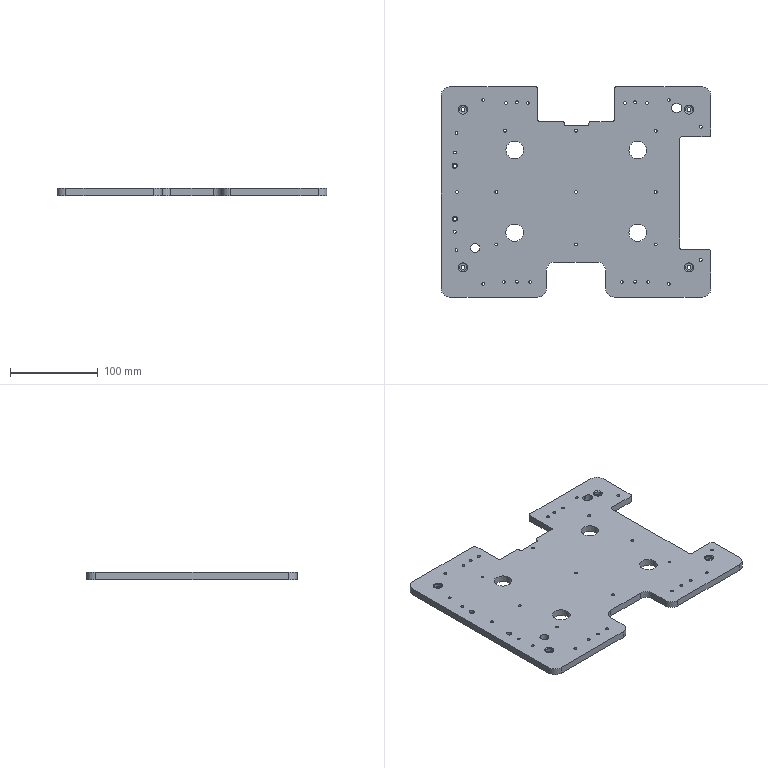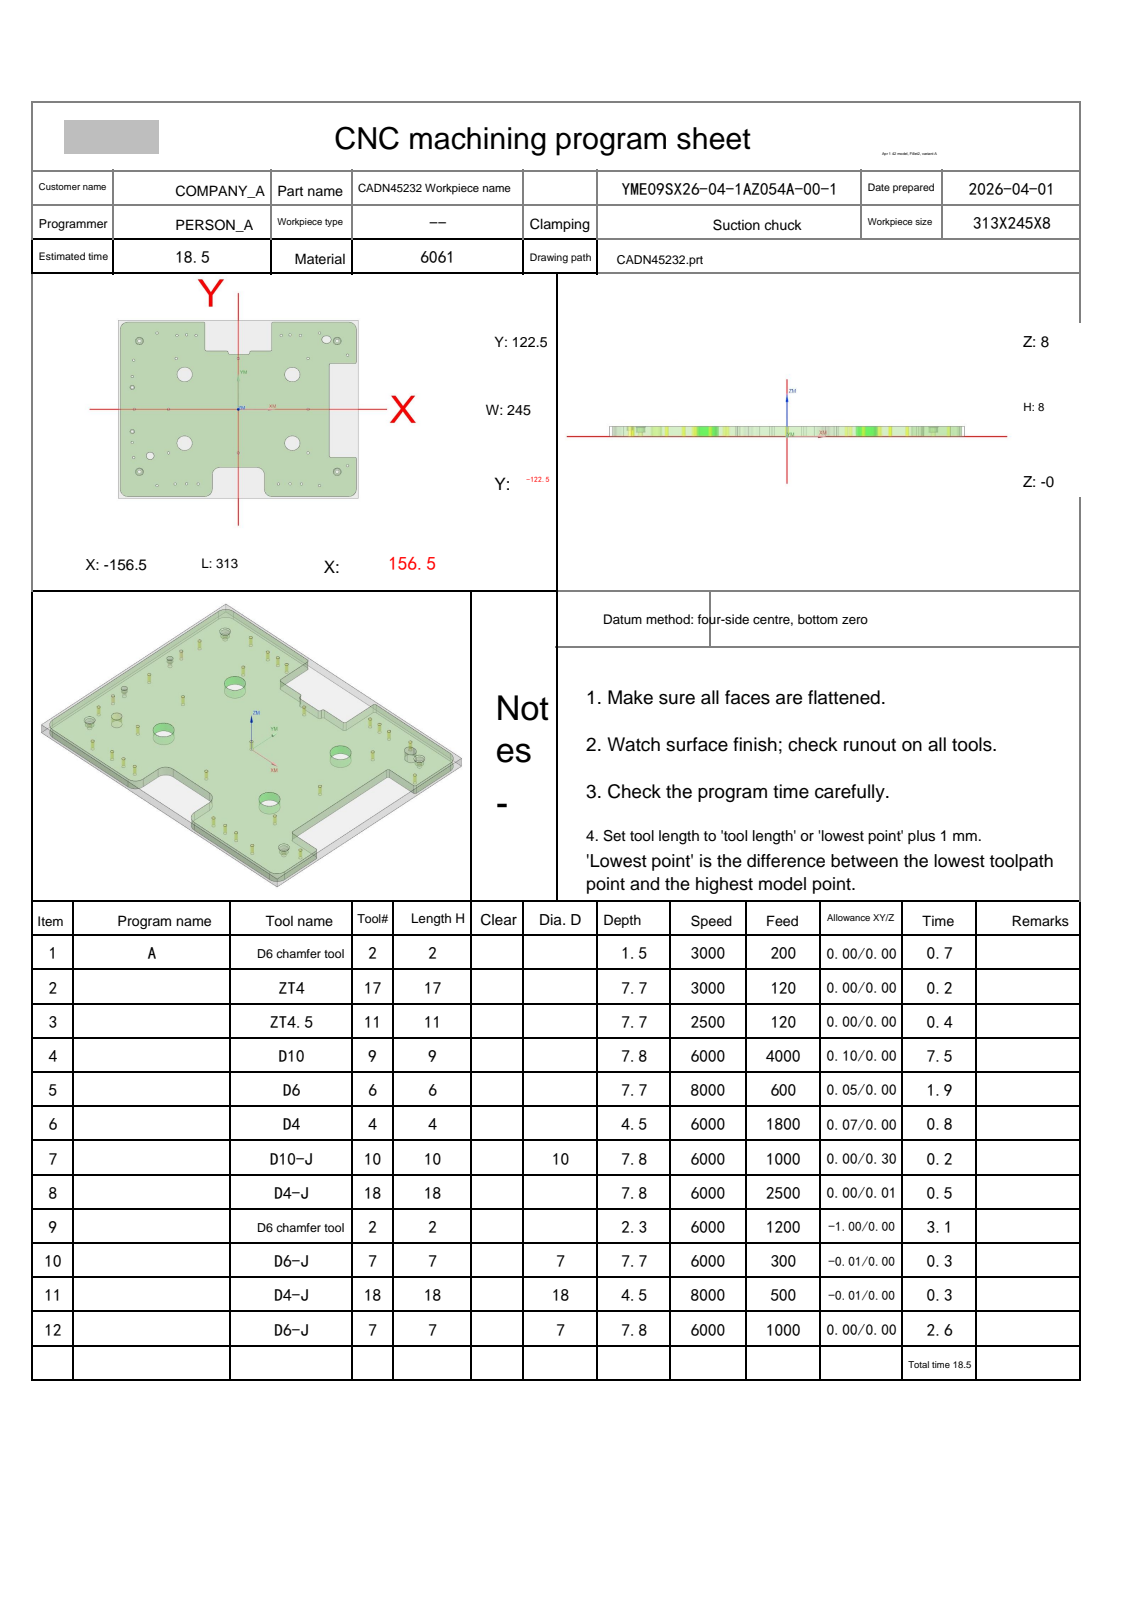NC program | NX | posted by the shop | part box 308 x 240 x 8 mm
Lines 1 to 1898 of 6786, first 1450 of 1896 lines:
%
O0001
(Machine time: 20.76 MIN)
(===Total Tool:9===)
(T2=D6 chamfer tool   D=6.   R=0.   D-  H02 Z=5.7   )
(T17=ZT4    D=4.   DR_a=118 D-  H17 Z=0.3   )
(T11=ZT4.5  D=4.5  DR_a=118 D-  H11 Z=0.3   )
(T9=D10     D=10.  R=0.   D-  H09 Z=0.2   )
(T6=D6      D=6.   R=0.   D-  H06 Z=0.3   )
(T4=D4      D=4.   R=0.   D-  H04 Z=3.5   )
(T10=D10-J  D=10.  R=0.   D10 H10 Z=0.2   )
(T18=D4-J   D=4.   R=0.   D-  H18 Z=0.2   )
(T7=D6-J    D=6.   R=0.   D7  H07 Z=0.2   )
G80 G90 G17 G49 G40
G91 G28 Z0
M01
N1 T02 M06
(D6 chamfer tool  D=6. R=0. H=02 ce=0.00 di=0.00)
G00 G90 G54 X-91. Y0.0 M03 S3000
G43 H02 Z28.
M08
G98 G81 X-91. Y0.0 Z6.5 R9. F200.
X-70.105 Y-46.566
X-91. Y-60.
X-52.35 Y-102.765
X-67.5 Y-102.5
X-82.35 Y-102.765
X-106. Y-105.
X-129. Y-85.991
X-115. Y-63.991
X-136.5 Y-66.5
X-138.327 Y-45.597
Y-30.597
X-135.8 Y0.0
X-138.327 Y30.083
Y45.083
X-136.5 Y67.5
X-129. Y94.009
X-106. Y105.
X-80. Y101.6
X-67.5 Y102.5
X-55. Y101.6
X-81. Y70.
X-70. Y48.
X0.0 Y70.
Y0.0
Y-60.
X52.35 Y-102.765
X67.5 Y-102.5
X82.35 Y-102.765
X106. Y-105.
X129. Y-85.991
X142.5 Y-77.5
X91. Y-60.
X70.458 Y-46.566
X91. Y0.0
X70.458 Y47.847
X91. Y70.
X56. Y101.6
X67.5 Y102.5
X81. Y101.6
X106. Y105.
X129. Y94.009
X142.5 Y74.508
G80
G00 Z28.
G91 G28 Z0.0
M05
M09
G91 G28 Z0.0
M01
N2 T17 M06
(ZT4 D=4. DR_a=118 H=17)
G00 G90 G54 X-138.327 Y30.083 M03 S3000
G43 H17 Z28.
M08
G98 G83 X-138.327 Y30.083 Z.3 R9. F120. Q3.
Y-30.597
G80
G00 Z28.
G91 G28 Z0.0
M05
M09
G91 G28 Z0.0
M01
N3 T11 M06
(ZT4.5 D=4.5 DR_a=118 H=11)
G00 G90 G54 X-129. Y94.009 M03 S2500
G43 H11 Z28.
M08
G98 G83 X-129. Y94.009 Z.3 R9. F120. Q3.
Y-85.991
X129.
Y94.009
G80
G00 Z28.
G91 G28 Z0.0
M05
M09
G91 G28 Z0.0
M01
N4 T09 M06
(D10  D=10. R=0. H=09 ce=0.10 di=0.30)
G00 G90 G54 X70.458 Y-46.566 M03 S6000
G43 H09 Z28.
M08
Z8.5
G03 X72.458 Y-48.566 I2. J0.0 F2700.
X74.458 Y-46.566 I0.0 J2.
X74.458 Y-46.566 Z8.3 I-4. J0.0 F3000.
X74.458 Y-46.566 Z8.1 I-4. J0.0
X74.458 Y-46.566 Z7.9 I-4. J0.0
X74.458 Y-46.566 Z7.7 I-4. J0.0
X74.458 Y-46.566 Z7.5 I-4. J0.0
X74.458 Y-46.566 Z7.3 I-4. J0.0
X74.458 Y-46.566 Z7.1 I-4. J0.0
X74.458 Y-46.566 Z6.9 I-4. J0.0
X74.458 Y-46.566 Z6.7 I-4. J0.0
X74.458 Y-46.566 Z6.5 I-4. J0.0
X74.458 Y-46.566 Z6.3 I-4. J0.0
X74.458 Y-46.566 Z6.1 I-4. J0.0
X74.458 Y-46.566 Z5.9 I-4. J0.0
X74.458 Y-46.566 Z5.7 I-4. J0.0
X74.458 Y-46.566 Z5.5 I-4. J0.0
X74.458 Y-46.566 Z5.3 I-4. J0.0
X74.458 Y-46.566 Z5.1 I-4. J0.0
X74.458 Y-46.566 Z4.9 I-4. J0.0
X74.458 Y-46.566 Z4.7 I-4. J0.0
X74.458 Y-46.566 Z4.5 I-4. J0.0
X74.458 Y-46.566 Z4.3 I-4. J0.0
X74.458 Y-46.566 Z4.1 I-4. J0.0
X74.458 Y-46.566 Z3.9 I-4. J0.0
X74.458 Y-46.566 Z3.7 I-4. J0.0
X74.458 Y-46.566 Z3.5 I-4. J0.0
X74.458 Y-46.566 Z3.3 I-4. J0.0
X74.458 Y-46.566 Z3.1 I-4. J0.0
X74.458 Y-46.566 Z2.9 I-4. J0.0
X74.458 Y-46.566 Z2.7 I-4. J0.0
X74.458 Y-46.566 Z2.5 I-4. J0.0
X74.458 Y-46.566 Z2.3 I-4. J0.0
X74.458 Y-46.566 Z2.1 I-4. J0.0
X74.458 Y-46.566 Z1.9 I-4. J0.0
X74.458 Y-46.566 Z1.7 I-4. J0.0
X74.458 Y-46.566 Z1.5 I-4. J0.0
X74.458 Y-46.566 Z1.3 I-4. J0.0
X74.458 Y-46.566 Z1.1 I-4. J0.0
X74.458 Y-46.566 Z.9 I-4. J0.0
X74.458 Y-46.566 Z.7 I-4. J0.0
X74.458 Y-46.566 Z.5 I-4. J0.0
X74.458 Y-46.566 Z.3 I-4. J0.0
X66.458 Y-46.566 Z.2 I-4. J0.0
X69.894 Y-50.607 I4.094 J0.0
X70.56 Y-50.661 I.666 J4.09
X74.476 Y-47.872 I0.0 J4.144
X74.711 Y-46.478 I-4.03 J1.394
X72.452 Y-42.714 I-4.264 J0.0
X70.378 Y-42.196 I-2.073 J-3.891
X66.858 Y-43.951 I0.0 J-4.409
X65.953 Y-46.654 I3.584 J-2.703
X67.213 Y-49.773 I4.489 J0.0
X70.546 Y-51.188 I3.334 J3.219
X73.206 Y-50.348 I0.0 J4.634
X75.232 Y-46.455 I-2.729 J3.894
X74.722 Y-44.312 I-4.755 J0.0
X70.43 Y-41.671 I-4.292 J-2.167
X68.944 Y-41.906 I0.0 J-4.808
X65.558 Y-46.566 I1.514 J-4.66
X70.458 Y-51.466 I4.9 J0.0
X75.358 Y-46.566 I0.0 J4.9
X70.458 Y-41.666 I-4.9 J0.0
X68.477 Y-42.085 I0.0 J-4.9
X67.018 Y-44.325 I.991 J-2.241
X69.468 Y-46.775 I2.45 J0.0
X70.458 Y-46.566 I0.0 J2.45
G00 Z28.
Y47.847
Z8.5
G03 X72.458 Y45.847 I2. J0.0 F2700.
X74.458 Y47.847 I0.0 J2.
X74.458 Y47.847 Z8.3 I-4. J0.0 F3000.
X74.458 Y47.847 Z8.1 I-4. J0.0
X74.458 Y47.847 Z7.9 I-4. J0.0
X74.458 Y47.847 Z7.7 I-4. J0.0
X74.458 Y47.847 Z7.5 I-4. J0.0
X74.458 Y47.847 Z7.3 I-4. J0.0
X74.458 Y47.847 Z7.1 I-4. J0.0
X74.458 Y47.847 Z6.9 I-4. J0.0
X74.458 Y47.847 Z6.7 I-4. J0.0
X74.458 Y47.847 Z6.5 I-4. J0.0
X74.458 Y47.847 Z6.3 I-4. J0.0
X74.458 Y47.847 Z6.1 I-4. J0.0
X74.458 Y47.847 Z5.9 I-4. J0.0
X74.458 Y47.847 Z5.7 I-4. J0.0
X74.458 Y47.847 Z5.5 I-4. J0.0
X74.458 Y47.847 Z5.3 I-4. J0.0
X74.458 Y47.847 Z5.1 I-4. J0.0
X74.458 Y47.847 Z4.9 I-4. J0.0
X74.458 Y47.847 Z4.7 I-4. J0.0
X74.458 Y47.847 Z4.5 I-4. J0.0
X74.458 Y47.847 Z4.3 I-4. J0.0
X74.458 Y47.847 Z4.1 I-4. J0.0
X74.458 Y47.847 Z3.9 I-4. J0.0
X74.458 Y47.847 Z3.7 I-4. J0.0
X74.458 Y47.847 Z3.5 I-4. J0.0
X74.458 Y47.847 Z3.3 I-4. J0.0
X74.458 Y47.847 Z3.1 I-4. J0.0
X74.458 Y47.847 Z2.9 I-4. J0.0
X74.458 Y47.847 Z2.7 I-4. J0.0
X74.458 Y47.847 Z2.5 I-4. J0.0
X74.458 Y47.847 Z2.3 I-4. J0.0
X74.458 Y47.847 Z2.1 I-4. J0.0
X74.458 Y47.847 Z1.9 I-4. J0.0
X74.458 Y47.847 Z1.7 I-4. J0.0
X74.458 Y47.847 Z1.5 I-4. J0.0
X74.458 Y47.847 Z1.3 I-4. J0.0
X74.458 Y47.847 Z1.1 I-4. J0.0
X74.458 Y47.847 Z.9 I-4. J0.0
X74.458 Y47.847 Z.7 I-4. J0.0
X74.458 Y47.847 Z.5 I-4. J0.0
X74.458 Y47.847 Z.3 I-4. J0.0
X66.458 Y47.847 Z.2 I-4. J0.0
X69.894 Y43.806 I4.094 J0.0
X70.56 Y43.752 I.666 J4.09
X74.476 Y46.541 I0.0 J4.144
X74.711 Y47.935 I-4.03 J1.394
X72.452 Y51.699 I-4.264 J0.0
X70.378 Y52.217 I-2.073 J-3.891
X66.858 Y50.462 I0.0 J-4.409
X65.953 Y47.759 I3.584 J-2.703
X67.213 Y44.64 I4.489 J0.0
X70.546 Y43.225 I3.334 J3.219
X73.206 Y44.065 I0.0 J4.634
X75.232 Y47.958 I-2.729 J3.894
X74.722 Y50.101 I-4.755 J0.0
X70.43 Y52.742 I-4.292 J-2.167
X68.944 Y52.507 I0.0 J-4.808
X65.558 Y47.847 I1.514 J-4.66
X70.458 Y42.947 I4.9 J0.0
X75.358 Y47.847 I0.0 J4.9
X70.458 Y52.747 I-4.9 J0.0
X68.477 Y52.328 I0.0 J-4.9
X67.018 Y50.088 I.991 J-2.241
X69.468 Y47.638 I2.45 J0.0
X70.458 Y47.847 I0.0 J2.45
G00 Z28.
X-70. Y48.
Z8.5
G03 X-68. Y46. I2. J0.0 F2700.
X-66. Y48. I0.0 J2.
X-66. Y48. Z8.3 I-4. J0.0 F3000.
X-66. Y48. Z8.1 I-4. J0.0
X-66. Y48. Z7.9 I-4. J0.0
X-66. Y48. Z7.7 I-4. J0.0
X-66. Y48. Z7.5 I-4. J0.0
X-66. Y48. Z7.3 I-4. J0.0
X-66. Y48. Z7.1 I-4. J0.0
X-66. Y48. Z6.9 I-4. J0.0
X-66. Y48. Z6.7 I-4. J0.0
X-66. Y48. Z6.5 I-4. J0.0
X-66. Y48. Z6.3 I-4. J0.0
X-66. Y48. Z6.1 I-4. J0.0
X-66. Y48. Z5.9 I-4. J0.0
X-66. Y48. Z5.7 I-4. J0.0
X-66. Y48. Z5.5 I-4. J0.0
X-66. Y48. Z5.3 I-4. J0.0
X-66. Y48. Z5.1 I-4. J0.0
X-66. Y48. Z4.9 I-4. J0.0
X-66. Y48. Z4.7 I-4. J0.0
X-66. Y48. Z4.5 I-4. J0.0
X-66. Y48. Z4.3 I-4. J0.0
X-66. Y48. Z4.1 I-4. J0.0
X-66. Y48. Z3.9 I-4. J0.0
X-66. Y48. Z3.7 I-4. J0.0
X-66. Y48. Z3.5 I-4. J0.0
X-66. Y48. Z3.3 I-4. J0.0
X-66. Y48. Z3.1 I-4. J0.0
X-66. Y48. Z2.9 I-4. J0.0
X-66. Y48. Z2.7 I-4. J0.0
X-66. Y48. Z2.5 I-4. J0.0
X-66. Y48. Z2.3 I-4. J0.0
X-66. Y48. Z2.1 I-4. J0.0
X-66. Y48. Z1.9 I-4. J0.0
X-66. Y48. Z1.7 I-4. J0.0
X-66. Y48. Z1.5 I-4. J0.0
X-66. Y48. Z1.3 I-4. J0.0
X-66. Y48. Z1.1 I-4. J0.0
X-66. Y48. Z.9 I-4. J0.0
X-66. Y48. Z.7 I-4. J0.0
X-66. Y48. Z.5 I-4. J0.0
X-66. Y48. Z.3 I-4. J0.0
X-74. Y48. Z.2 I-4. J0.0
X-70.564 Y43.959 I4.094 J0.0
X-69.898 Y43.905 I.666 J4.09
X-65.982 Y46.694 I0.0 J4.144
X-65.748 Y48.088 I-4.03 J1.394
X-68.007 Y51.852 I-4.264 J0.0
X-70.08 Y52.37 I-2.073 J-3.891
X-73.6 Y50.616 I0.0 J-4.409
X-74.505 Y47.912 I3.584 J-2.703
X-73.245 Y44.794 I4.489 J0.0
X-69.912 Y43.379 I3.334 J3.219
X-67.252 Y44.218 I0.0 J4.634
X-65.226 Y48.112 I-2.729 J3.894
X-65.736 Y50.254 I-4.755 J0.0
X-70.028 Y52.896 I-4.292 J-2.167
X-71.514 Y52.66 I0.0 J-4.808
X-74.9 Y48. I1.514 J-4.66
X-70. Y43.1 I4.9 J0.0
X-65.1 Y48. I0.0 J4.9
X-70. Y52.9 I-4.9 J0.0
X-71.981 Y52.482 I0.0 J-4.9
X-73.441 Y50.241 I.991 J-2.241
X-70.991 Y47.791 I2.45 J0.0
X-70. Y48. I0.0 J2.45
G00 Z28.
X-70.105 Y-46.566
Z8.5
G03 X-68.105 Y-48.566 I2. J0.0 F2700.
X-66.105 Y-46.566 I0.0 J2.
X-66.105 Y-46.566 Z8.3 I-4. J0.0 F3000.
X-66.105 Y-46.566 Z8.1 I-4. J0.0
X-66.105 Y-46.566 Z7.9 I-4. J0.0
X-66.105 Y-46.566 Z7.7 I-4. J0.0
X-66.105 Y-46.566 Z7.5 I-4. J0.0
X-66.105 Y-46.566 Z7.3 I-4. J0.0
X-66.105 Y-46.566 Z7.1 I-4. J0.0
X-66.105 Y-46.566 Z6.9 I-4. J0.0
X-66.105 Y-46.566 Z6.7 I-4. J0.0
X-66.105 Y-46.566 Z6.5 I-4. J0.0
X-66.105 Y-46.566 Z6.3 I-4. J0.0
X-66.105 Y-46.566 Z6.1 I-4. J0.0
X-66.105 Y-46.566 Z5.9 I-4. J0.0
X-66.105 Y-46.566 Z5.7 I-4. J0.0
X-66.105 Y-46.566 Z5.5 I-4. J0.0
X-66.105 Y-46.566 Z5.3 I-4. J0.0
X-66.105 Y-46.566 Z5.1 I-4. J0.0
X-66.105 Y-46.566 Z4.9 I-4. J0.0
X-66.105 Y-46.566 Z4.7 I-4. J0.0
X-66.105 Y-46.566 Z4.5 I-4. J0.0
X-66.105 Y-46.566 Z4.3 I-4. J0.0
X-66.105 Y-46.566 Z4.1 I-4. J0.0
X-66.105 Y-46.566 Z3.9 I-4. J0.0
X-66.105 Y-46.566 Z3.7 I-4. J0.0
X-66.105 Y-46.566 Z3.5 I-4. J0.0
X-66.105 Y-46.566 Z3.3 I-4. J0.0
X-66.105 Y-46.566 Z3.1 I-4. J0.0
X-66.105 Y-46.566 Z2.9 I-4. J0.0
X-66.105 Y-46.566 Z2.7 I-4. J0.0
X-66.105 Y-46.566 Z2.5 I-4. J0.0
X-66.105 Y-46.566 Z2.3 I-4. J0.0
X-66.105 Y-46.566 Z2.1 I-4. J0.0
X-66.105 Y-46.566 Z1.9 I-4. J0.0
X-66.105 Y-46.566 Z1.7 I-4. J0.0
X-66.105 Y-46.566 Z1.5 I-4. J0.0
X-66.105 Y-46.566 Z1.3 I-4. J0.0
X-66.105 Y-46.566 Z1.1 I-4. J0.0
X-66.105 Y-46.566 Z.9 I-4. J0.0
X-66.105 Y-46.566 Z.7 I-4. J0.0
X-66.105 Y-46.566 Z.5 I-4. J0.0
X-66.105 Y-46.566 Z.3 I-4. J0.0
X-74.105 Y-46.566 Z.2 I-4. J0.0
X-70.669 Y-50.607 I4.094 J0.0
X-70.003 Y-50.661 I.666 J4.09
X-66.087 Y-47.872 I0.0 J4.144
X-65.852 Y-46.478 I-4.03 J1.394
X-68.111 Y-42.714 I-4.264 J0.0
X-70.185 Y-42.196 I-2.073 J-3.891
X-73.705 Y-43.951 I0.0 J-4.409
X-74.61 Y-46.654 I3.584 J-2.703
X-73.35 Y-49.773 I4.489 J0.0
X-70.017 Y-51.188 I3.334 J3.219
X-67.357 Y-50.348 I0.0 J4.634
X-65.331 Y-46.455 I-2.729 J3.894
X-65.841 Y-44.312 I-4.755 J0.0
X-70.133 Y-41.671 I-4.292 J-2.167
X-71.619 Y-41.906 I0.0 J-4.808
X-75.005 Y-46.566 I1.514 J-4.66
X-70.105 Y-51.466 I4.9 J0.0
X-65.205 Y-46.566 I0.0 J4.9
X-70.105 Y-41.666 I-4.9 J0.0
X-72.086 Y-42.085 I0.0 J-4.9
X-73.545 Y-44.325 I.991 J-2.241
X-71.095 Y-46.775 I2.45 J0.0
X-70.105 Y-46.566 I0.0 J2.45
G00 Z28.
G00 G90 X-159.1 Y0.0 M03 S6000
Z28.
Z8.5
G01 Y110. Z8.461 F4000.
G02 X-144. Y125.1 Z8.452 I15.1 J0.0
G01 X-45.5 Z8.417
G02 X-38.4 Y118. Z8.413 I0.0 J-7.1
G01 Y85.389 Z8.401
X-14.961 Z8.393
X-13.8 Y85.272 Z8.392
X-12.44 Y84.851
X-11.191 Y84.169 Z8.391
X-10.103 Y83.251
X-9.219 Y82.136 Z8.39
X-8.574 Y80.868
X-8.557 Y80.806
X10.141 Z8.383
X10.221 Y81.063
X10.903 Y82.312
X11.82 Y83.401 Z8.382
X12.935 Y84.285
X14.203 Y84.931 Z8.381
X15.538 Y85.301
X16.566 Y85.389 Z8.38
X38.4 Z8.372
Y118. Z8.361
G02 X45.5 Y125.1 Z8.357 I7.1 J0.0
G01 X144. Z8.322
G02 X159.1 Y110. Z8.313 I0.0 J-15.1
G01 Y65.004 Z8.297
G02 X152. Y57.904 Z8.293 I-7.1 J0.0
G01 X123.763 Z8.283
Y-60.896 Z8.24
X152. Z8.23
G02 X159.1 Y-67.996 Z8.226 I0.0 J-7.1
G01 Y-110. Z8.211
G02 X144. Y-125.1 Z8.203 I-15.1 J0.0
G01 X44. Z8.167
G02 X28.9 Y-110. Z8.158 I0.0 J15.1
G01 Y-90. Z8.151
G03 X24. Y-85.1 Z8.149 I-4.9 J0.0
G01 X-24. Z8.131
G03 X-28.9 Y-90. Z8.129 I0.0 J-4.9
G01 Y-110. Z8.122
G02 X-44. Y-125.1 Z8.113 I-15.1 J0.0
G01 X-144. Z8.077
G02 X-159.1 Y-110. Z8.069 I0.0 J15.1
G01 Y110. Z7.99
G02 X-144. Y125.1 Z7.982 I15.1 J0.0
G01 X-45.5 Z7.946
G02 X-38.4 Y118. Z7.942 I0.0 J-7.1
G01 Y85.389 Z7.931
X-14.961 Z7.922
X-13.8 Y85.272
X-12.44 Y84.851 Z7.921
X-11.191 Y84.169
X-10.103 Y83.251 Z7.92
X-9.219 Y82.136
X-8.574 Y80.868 Z7.919
X-8.557 Y80.806
X10.141 Z7.913
X10.221 Y81.063
X10.903 Y82.312 Z7.912
X11.82 Y83.401
X12.935 Y84.285 Z7.911
X14.203 Y84.931 Z7.91
X15.538 Y85.301
X16.566 Y85.389
X38.4 Z7.902
Y118. Z7.89
G02 X45.5 Y125.1 Z7.886 I7.1 J0.0
G01 X144. Z7.851
G02 X159.1 Y110. Z7.842 I0.0 J-15.1
G01 Y65.004 Z7.826
G02 X152. Y57.904 Z7.822 I-7.1 J0.0
G01 X123.763 Z7.812
Y-60.896 Z7.77
X152. Z7.76
G02 X159.1 Y-67.996 Z7.756 I0.0 J-7.1
G01 Y-110. Z7.741
G02 X144. Y-125.1 Z7.732 I-15.1 J0.0
G01 X44. Z7.696
G02 X28.9 Y-110. Z7.688 I0.0 J15.1
G01 Y-90. Z7.681
G03 X24. Y-85.1 Z7.678 I-4.9 J0.0
G01 X-24. Z7.661
G03 X-28.9 Y-90. Z7.658 I0.0 J-4.9
G01 Y-110. Z7.651
G02 X-44. Y-125.1 Z7.642 I-15.1 J0.0
G01 X-144. Z7.607
G02 X-159.1 Y-110. Z7.598 I0.0 J15.1
G01 Y110. Z7.519
G02 X-144. Y125.1 Z7.511 I15.1 J0.0
G01 X-45.5 Z7.476
G02 X-38.4 Y118. Z7.472 I0.0 J-7.1
G01 Y85.389 Z7.46
X-14.961 Z7.452
X-13.8 Y85.272 Z7.451
X-12.44 Y84.851
X-11.191 Y84.169 Z7.45
X-10.103 Y83.251
X-9.219 Y82.136 Z7.449
X-8.574 Y80.868
X-8.557 Y80.806
X10.141 Z7.442
X10.221 Y81.063
X10.903 Y82.312 Z7.441
X11.82 Y83.401
X12.935 Y84.285 Z7.44
X14.203 Y84.931
X15.538 Y85.301 Z7.439
X16.566 Y85.389
X38.4 Z7.431
Y118. Z7.42
G02 X45.5 Y125.1 Z7.416 I7.1 J0.0
G01 X144. Z7.38
G02 X159.1 Y110. Z7.372 I0.0 J-15.1
G01 Y65.004 Z7.356
G02 X152. Y57.904 Z7.352 I-7.1 J0.0
G01 X123.763 Z7.342
Y-60.896 Z7.299
X152. Z7.289
G02 X159.1 Y-67.996 Z7.285 I0.0 J-7.1
G01 Y-110. Z7.27
G02 X144. Y-125.1 Z7.262 I-15.1 J0.0
G01 X44. Z7.226
G02 X28.9 Y-110. Z7.217 I0.0 J15.1
G01 Y-90. Z7.21
G03 X24. Y-85.1 Z7.207 I-4.9 J0.0
G01 X-24. Z7.19
G03 X-28.9 Y-90. Z7.187 I0.0 J-4.9
G01 Y-110. Z7.18
G02 X-44. Y-125.1 Z7.172 I-15.1 J0.0
G01 X-144. Z7.136
G02 X-159.1 Y-110. Z7.128 I0.0 J15.1
G01 Y110. Z7.049
G02 X-144. Y125.1 Z7.04 I15.1 J0.0
G01 X-45.5 Z7.005
G02 X-38.4 Y118. Z7.001 I0.0 J-7.1
G01 Y85.389 Z6.99
X-14.961 Z6.981
X-13.8 Y85.272
X-12.44 Y84.851 Z6.98
X-11.191 Y84.169
X-10.103 Y83.251 Z6.979
X-9.219 Y82.136
X-8.574 Y80.868 Z6.978
X-8.557 Y80.806
X10.141 Z6.971
X10.221 Y81.063
X10.903 Y82.312
X11.82 Y83.401 Z6.97
X12.935 Y84.285
X14.203 Y84.931 Z6.969
X15.538 Y85.301
X16.566 Y85.389 Z6.968
X38.4 Z6.961
Y118. Z6.949
G02 X45.5 Y125.1 Z6.945 I7.1 J0.0
G01 X144. Z6.91
G02 X159.1 Y110. Z6.901 I0.0 J-15.1
G01 Y65.004 Z6.885
G02 X152. Y57.904 Z6.881 I-7.1 J0.0
G01 X123.763 Z6.871
Y-60.896 Z6.829
X152. Z6.818
G02 X159.1 Y-67.996 Z6.814 I0.0 J-7.1
G01 Y-110. Z6.799
G02 X144. Y-125.1 Z6.791 I-15.1 J0.0
G01 X44. Z6.755
G02 X28.9 Y-110. Z6.747 I0.0 J15.1
G01 Y-90. Z6.74
G03 X24. Y-85.1 Z6.737 I-4.9 J0.0
G01 X-24. Z6.72
G03 X-28.9 Y-90. Z6.717 I0.0 J-4.9
G01 Y-110. Z6.71
G02 X-44. Y-125.1 Z6.701 I-15.1 J0.0
G01 X-144. Z6.665
G02 X-159.1 Y-110. Z6.657 I0.0 J15.1
G01 Y110. Z6.578
G02 X-144. Y125.1 Z6.57 I15.1 J0.0
G01 X-45.5 Z6.535
G02 X-38.4 Y118. Z6.531 I0.0 J-7.1
G01 Y85.389 Z6.519
X-14.961 Z6.511
X-13.8 Y85.272 Z6.51
X-12.44 Y84.851
X-11.191 Y84.169 Z6.509
X-10.103 Y83.251
X-9.219 Y82.136 Z6.508
X-8.574 Y80.868
X-8.557 Y80.806
X10.141 Z6.501
X10.221 Y81.063
X10.903 Y82.312 Z6.5
X11.82 Y83.401
X12.935 Y84.285 Z6.499
X14.203 Y84.931
X15.538 Y85.301 Z6.498
X16.566 Y85.389
X38.4 Z6.49
Y118. Z6.478
G02 X45.5 Y125.1 Z6.474 I7.1 J0.0
G01 X144. Z6.439
G02 X159.1 Y110. Z6.431 I0.0 J-15.1
G01 Y65.004 Z6.415
G02 X152. Y57.904 Z6.411 I-7.1 J0.0
G01 X123.763 Z6.4
Y-60.896 Z6.358
X152. Z6.348
G02 X159.1 Y-67.996 Z6.344 I0.0 J-7.1
G01 Y-110. Z6.329
G02 X144. Y-125.1 Z6.32 I-15.1 J0.0
G01 X44. Z6.285
G02 X28.9 Y-110. Z6.276 I0.0 J15.1
G01 Y-90. Z6.269
G03 X24. Y-85.1 Z6.266 I-4.9 J0.0
G01 X-24. Z6.249
G03 X-28.9 Y-90. Z6.246 I0.0 J-4.9
G01 Y-110. Z6.239
G02 X-44. Y-125.1 Z6.231 I-15.1 J0.0
G01 X-144. Z6.195
G02 X-159.1 Y-110. Z6.186 I0.0 J15.1
G01 Y110. Z6.108
G02 X-144. Y125.1 Z6.099 I15.1 J0.0
G01 X-45.5 Z6.064
G02 X-38.4 Y118. Z6.06 I0.0 J-7.1
G01 Y85.389 Z6.048
X-14.961 Z6.04
X-13.8 Y85.272
X-12.44 Y84.851 Z6.039
X-11.191 Y84.169
X-10.103 Y83.251 Z6.038
X-9.219 Y82.136 Z6.037
X-8.574 Y80.868
X-8.557 Y80.806
X10.141 Z6.03
X10.221 Y81.063
X10.903 Y82.312
X11.82 Y83.401 Z6.029
X12.935 Y84.285
X14.203 Y84.931 Z6.028
X15.538 Y85.301
X16.566 Y85.389 Z6.027
X38.4 Z6.019
Y118. Z6.008
G02 X45.5 Y125.1 Z6.004 I7.1 J0.0
G01 X144. Z5.969
G02 X159.1 Y110. Z5.96 I0.0 J-15.1
G01 Y65.004 Z5.944
G02 X152. Y57.904 Z5.94 I-7.1 J0.0
G01 X123.763 Z5.93
Y-60.896 Z5.887
X152. Z5.877
G02 X159.1 Y-67.996 Z5.873 I0.0 J-7.1
G01 Y-110. Z5.858
G02 X144. Y-125.1 Z5.85 I-15.1 J0.0
G01 X44. Z5.814
G02 X28.9 Y-110. Z5.806 I0.0 J15.1
G01 Y-90. Z5.798
G03 X24. Y-85.1 Z5.796 I-4.9 J0.0
G01 X-24. Z5.778
G03 X-28.9 Y-90. Z5.776 I0.0 J-4.9
G01 Y-110. Z5.769
G02 X-44. Y-125.1 Z5.76 I-15.1 J0.0
G01 X-144. Z5.724
G02 X-159.1 Y-110. Z5.716 I0.0 J15.1
G01 Y110. Z5.637
G02 X-144. Y125.1 Z5.629 I15.1 J0.0
G01 X-45.5 Z5.593
G02 X-38.4 Y118. Z5.589 I0.0 J-7.1
G01 Y85.389 Z5.578
X-14.961 Z5.569
X-13.8 Y85.272
X-12.44 Y84.851 Z5.568
X-11.191 Y84.169
X-10.103 Y83.251 Z5.567
X-9.219 Y82.136
X-8.574 Y80.868 Z5.566
X-8.557 Y80.806
X10.141 Z5.56
X10.221 Y81.063
X10.903 Y82.312 Z5.559
X11.82 Y83.401
X12.935 Y84.285 Z5.558
X14.203 Y84.931
X15.538 Y85.301 Z5.557
X16.566 Y85.389
X38.4 Z5.549
Y118. Z5.537
G02 X45.5 Y125.1 Z5.533 I7.1 J0.0
G01 X144. Z5.498
G02 X159.1 Y110. Z5.49 I0.0 J-15.1
G01 Y65.004 Z5.473
G02 X152. Y57.904 Z5.469 I-7.1 J0.0
G01 X123.763 Z5.459
Y-60.896 Z5.417
X152. Z5.407
G02 X159.1 Y-67.996 Z5.403 I0.0 J-7.1
G01 Y-110. Z5.388
G02 X144. Y-125.1 Z5.379 I-15.1 J0.0
G01 X44. Z5.343
G02 X28.9 Y-110. Z5.335 I0.0 J15.1
G01 Y-90. Z5.328
G03 X24. Y-85.1 Z5.325 I-4.9 J0.0
G01 X-24. Z5.308
G03 X-28.9 Y-90. Z5.305 I0.0 J-4.9
G01 Y-110. Z5.298
G02 X-44. Y-125.1 Z5.289 I-15.1 J0.0
G01 X-144. Z5.254
G02 X-159.1 Y-110. Z5.245 I0.0 J15.1
G01 Y110. Z5.167
G02 X-144. Y125.1 Z5.158 I15.1 J0.0
G01 X-45.5 Z5.123
G02 X-38.4 Y118. Z5.119 I0.0 J-7.1
G01 Y85.389 Z5.107
X-14.961 Z5.099
X-13.8 Y85.272 Z5.098
X-12.44 Y84.851
X-11.191 Y84.169 Z5.097
X-10.103 Y83.251
X-9.219 Y82.136 Z5.096
X-8.574 Y80.868
X-8.557 Y80.806
X10.141 Z5.089
X10.221 Y81.063
X10.903 Y82.312 Z5.088
X11.82 Y83.401
X12.935 Y84.285 Z5.087
X14.203 Y84.931
X15.538 Y85.301 Z5.086
X16.566 Y85.389
X38.4 Z5.078
Y118. Z5.067
G02 X45.5 Y125.1 Z5.063 I7.1 J0.0
G01 X144. Z5.027
G02 X159.1 Y110. Z5.019 I0.0 J-15.1
G01 Y65.004 Z5.003
G02 X152. Y57.904 Z4.999 I-7.1 J0.0
G01 X123.763 Z4.989
Y-60.896 Z4.946
X152. Z4.936
G02 X159.1 Y-67.996 Z4.932 I0.0 J-7.1
G01 Y-110. Z4.917
G02 X144. Y-125.1 Z4.909 I-15.1 J0.0
G01 X44. Z4.873
G02 X28.9 Y-110. Z4.864 I0.0 J15.1
G01 Y-90. Z4.857
G03 X24. Y-85.1 Z4.854 I-4.9 J0.0
G01 X-24. Z4.837
G03 X-28.9 Y-90. Z4.835 I0.0 J-4.9
G01 Y-110. Z4.827
G02 X-44. Y-125.1 Z4.819 I-15.1 J0.0
G01 X-144. Z4.783
G02 X-159.1 Y-110. Z4.775 I0.0 J15.1
G01 Y110. Z4.696
G02 X-144. Y125.1 Z4.687 I15.1 J0.0
G01 X-45.5 Z4.652
G02 X-38.4 Y118. Z4.648 I0.0 J-7.1
G01 Y85.389 Z4.637
X-14.961 Z4.628
X-13.8 Y85.272
X-12.44 Y84.851 Z4.627
X-11.191 Y84.169
X-10.103 Y83.251 Z4.626
X-9.219 Y82.136
X-8.574 Y80.868 Z4.625
X-8.557 Y80.806
X10.141 Z4.619
X10.221 Y81.063 Z4.618
X10.903 Y82.312
X11.82 Y83.401 Z4.617
X12.935 Y84.285
X14.203 Y84.931 Z4.616
X15.538 Y85.301
X16.566 Y85.389
X38.4 Z4.608
Y118. Z4.596
G02 X45.5 Y125.1 Z4.592 I7.1 J0.0
G01 X144. Z4.557
G02 X159.1 Y110. Z4.548 I0.0 J-15.1
G01 Y65.004 Z4.532
G02 X152. Y57.904 Z4.528 I-7.1 J0.0
G01 X123.763 Z4.518
Y-60.896 Z4.476
X152. Z4.466
G02 X159.1 Y-67.996 Z4.462 I0.0 J-7.1
G01 Y-110. Z4.447
G02 X144. Y-125.1 Z4.438 I-15.1 J0.0
G01 X44. Z4.402
G02 X28.9 Y-110. Z4.394 I0.0 J15.1
G01 Y-90. Z4.387
G03 X24. Y-85.1 Z4.384 I-4.9 J0.0
G01 X-24. Z4.367
G03 X-28.9 Y-90. Z4.364 I0.0 J-4.9
G01 Y-110. Z4.357
G02 X-44. Y-125.1 Z4.348 I-15.1 J0.0
G01 X-144. Z4.313
G02 X-159.1 Y-110. Z4.304 I0.0 J15.1
G01 Y110. Z4.225
G02 X-144. Y125.1 Z4.217 I15.1 J0.0
G01 X-45.5 Z4.182
G02 X-38.4 Y118. Z4.178 I0.0 J-7.1
G01 Y85.389 Z4.166
X-14.961 Z4.158
X-13.8 Y85.272 Z4.157
X-12.44 Y84.851
X-11.191 Y84.169 Z4.156
X-10.103 Y83.251
X-9.219 Y82.136 Z4.155
X-8.574 Y80.868
X-8.557 Y80.806
X10.141 Z4.148
X10.221 Y81.063
X10.903 Y82.312 Z4.147
X11.82 Y83.401
X12.935 Y84.285 Z4.146
X14.203 Y84.931
X15.538 Y85.301 Z4.145
X16.566 Y85.389
X38.4 Z4.137
Y118. Z4.125
G02 X45.5 Y125.1 Z4.121 I7.1 J0.0
G01 X144. Z4.086
G02 X159.1 Y110. Z4.078 I0.0 J-15.1
G01 Y65.004 Z4.062
G02 X152. Y57.904 Z4.058 I-7.1 J0.0
G01 X123.763 Z4.048
Y-60.896 Z4.005
X152. Z3.995
G02 X159.1 Y-67.996 Z3.991 I0.0 J-7.1
G01 Y-110. Z3.976
G02 X144. Y-125.1 Z3.967 I-15.1 J0.0
G01 X44. Z3.932
G02 X28.9 Y-110. Z3.923 I0.0 J15.1
G01 Y-90. Z3.916
G03 X24. Y-85.1 Z3.913 I-4.9 J0.0
G01 X-24. Z3.896
G03 X-28.9 Y-90. Z3.893 I0.0 J-4.9
G01 Y-110. Z3.886
G02 X-44. Y-125.1 Z3.878 I-15.1 J0.0
G01 X-144. Z3.842
G02 X-159.1 Y-110. Z3.833 I0.0 J15.1
G01 Y110. Z3.755
G02 X-144. Y125.1 Z3.746 I15.1 J0.0
G01 X-45.5 Z3.711
G02 X-38.4 Y118. Z3.707 I0.0 J-7.1
G01 Y85.389 Z3.695
X-14.961 Z3.687
X-13.8 Y85.272
X-12.44 Y84.851 Z3.686
X-11.191 Y84.169
X-10.103 Y83.251 Z3.685
X-9.219 Y82.136
X-8.574 Y80.868 Z3.684
X-8.557 Y80.806
X10.141 Z3.677
X10.221 Y81.063
X10.903 Y82.312
X11.82 Y83.401 Z3.676
X12.935 Y84.285
X14.203 Y84.931 Z3.675
X15.538 Y85.301
X16.566 Y85.389 Z3.674
X38.4 Z3.667
Y118. Z3.655
G02 X45.5 Y125.1 Z3.651 I7.1 J0.0
G01 X144. Z3.616
G02 X159.1 Y110. Z3.607 I0.0 J-15.1
G01 Y65.004 Z3.591
G02 X152. Y57.904 Z3.587 I-7.1 J0.0
G01 X123.763 Z3.577
Y-60.896 Z3.534
X152. Z3.524
G02 X159.1 Y-67.996 Z3.52 I0.0 J-7.1
G01 Y-110. Z3.505
G02 X144. Y-125.1 Z3.497 I-15.1 J0.0
G01 X44. Z3.461
G02 X28.9 Y-110. Z3.453 I0.0 J15.1
G01 Y-90. Z3.445
G03 X24. Y-85.1 Z3.443 I-4.9 J0.0
G01 X-24. Z3.426
G03 X-28.9 Y-90. Z3.423 I0.0 J-4.9
G01 Y-110. Z3.416
G02 X-44. Y-125.1 Z3.407 I-15.1 J0.0
G01 X-144. Z3.371
G02 X-159.1 Y-110. Z3.363 I0.0 J15.1
G01 Y110. Z3.284
G02 X-144. Y125.1 Z3.276 I15.1 J0.0
G01 X-45.5 Z3.24
G02 X-38.4 Y118. Z3.236 I0.0 J-7.1
G01 Y85.389 Z3.225
X-14.961 Z3.216
X-13.8 Y85.272
X-12.44 Y84.851 Z3.215
X-11.191 Y84.169
X-10.103 Y83.251 Z3.214
X-9.219 Y82.136
X-8.574 Y80.868 Z3.213
X-8.557 Y80.806
X10.141 Z3.207
X10.221 Y81.063
X10.903 Y82.312 Z3.206
X11.82 Y83.401
X12.935 Y84.285 Z3.205
X14.203 Y84.931
X15.538 Y85.301 Z3.204
X16.566 Y85.389
X38.4 Z3.196
Y118. Z3.184
G02 X45.5 Y125.1 Z3.18 I7.1 J0.0
G01 X144. Z3.145
G02 X159.1 Y110. Z3.137 I0.0 J-15.1
G01 Y65.004 Z3.12
G02 X152. Y57.904 Z3.116 I-7.1 J0.0
G01 X123.763 Z3.106
Y-60.896 Z3.064
X152. Z3.054
G02 X159.1 Y-67.996 Z3.05 I0.0 J-7.1
G01 Y-110. Z3.035
G02 X144. Y-125.1 Z3.026 I-15.1 J0.0
G01 X44. Z2.991
G02 X28.9 Y-110. Z2.982 I0.0 J15.1
G01 Y-90. Z2.975
G03 X24. Y-85.1 Z2.972 I-4.9 J0.0
G01 X-24. Z2.955
G03 X-28.9 Y-90. Z2.952 I0.0 J-4.9
G01 Y-110. Z2.945
G02 X-44. Y-125.1 Z2.937 I-15.1 J0.0
G01 X-144. Z2.901
G02 X-159.1 Y-110. Z2.892 I0.0 J15.1
G01 Y110. Z2.814
G02 X-144. Y125.1 Z2.805 I15.1 J0.0
G01 X-45.5 Z2.77
G02 X-38.4 Y118. Z2.766 I0.0 J-7.1
G01 Y85.389 Z2.754
X-14.961 Z2.746
X-13.8 Y85.272 Z2.745
X-12.44 Y84.851
X-11.191 Y84.169 Z2.744
X-10.103 Y83.251
X-9.219 Y82.136 Z2.743
X-8.574 Y80.868
X-8.557 Y80.806
X10.141 Z2.736
X10.221 Y81.063
X10.903 Y82.312
X11.82 Y83.401 Z2.735
X12.935 Y84.285
X14.203 Y84.931 Z2.734
X15.538 Y85.301
X16.566 Y85.389 Z2.733
X38.4 Z2.725
Y118. Z2.714
G02 X45.5 Y125.1 Z2.71 I7.1 J0.0
G01 X144. Z2.674
G02 X159.1 Y110. Z2.666 I0.0 J-15.1
G01 Y65.004 Z2.65
G02 X152. Y57.904 Z2.646 I-7.1 J0.0
G01 X123.763 Z2.636
Y-60.896 Z2.593
X152. Z2.583
G02 X159.1 Y-67.996 Z2.579 I0.0 J-7.1
G01 Y-110. Z2.564
G02 X144. Y-125.1 Z2.556 I-15.1 J0.0
G01 X44. Z2.52
G02 X28.9 Y-110. Z2.511 I0.0 J15.1
G01 Y-90. Z2.504
G03 X24. Y-85.1 Z2.502 I-4.9 J0.0
G01 X-24. Z2.484
G03 X-28.9 Y-90. Z2.482 I0.0 J-4.9
G01 Y-110. Z2.474
G02 X-44. Y-125.1 Z2.466 I-15.1 J0.0
G01 X-144. Z2.43
G02 X-159.1 Y-110. Z2.422 I0.0 J15.1
G01 Y110. Z2.343
G02 X-144. Y125.1 Z2.335 I15.1 J0.0
G01 X-45.5 Z2.299
G02 X-38.4 Y118. Z2.295 I0.0 J-7.1
G01 Y85.389 Z2.284
X-14.961 Z2.275
X-13.8 Y85.272
X-12.44 Y84.851 Z2.274
X-11.191 Y84.169
X-10.103 Y83.251 Z2.273
X-9.219 Y82.136
X-8.574 Y80.868 Z2.272
X-8.557 Y80.806
X10.141 Z2.266
X10.221 Y81.063 Z2.265
X10.903 Y82.312
X11.82 Y83.401 Z2.264
X12.935 Y84.285
X14.203 Y84.931 Z2.263
X15.538 Y85.301
X16.566 Y85.389
X38.4 Z2.255
Y118. Z2.243
G02 X45.5 Y125.1 Z2.239 I7.1 J0.0
G01 X144. Z2.204
G02 X159.1 Y110. Z2.195 I0.0 J-15.1
G01 Y65.004 Z2.179
G02 X152. Y57.904 Z2.175 I-7.1 J0.0
G01 X123.763 Z2.165
Y-60.896 Z2.123
X152. Z2.113
G02 X159.1 Y-67.996 Z2.109 I0.0 J-7.1
G01 Y-110. Z2.094
G02 X144. Y-125.1 Z2.085 I-15.1 J0.0
G01 X44. Z2.049
G02 X28.9 Y-110. Z2.041 I0.0 J15.1
G01 Y-90. Z2.034
G03 X24. Y-85.1 Z2.031 I-4.9 J0.0
G01 X-24. Z2.014
G03 X-28.9 Y-90. Z2.011 I0.0 J-4.9
G01 Y-110. Z2.004
G02 X-44. Y-125.1 Z1.995 I-15.1 J0.0
G01 X-144. Z1.96
G02 X-159.1 Y-110. Z1.951 I0.0 J15.1
G01 Y110. Z1.872
G02 X-144. Y125.1 Z1.864 I15.1 J0.0
G01 X-45.5 Z1.829
G02 X-38.4 Y118. Z1.825 I0.0 J-7.1
G01 Y85.389 Z1.813
X-14.961 Z1.805
X-13.8 Y85.272 Z1.804
X-12.44 Y84.851
X-11.191 Y84.169 Z1.803
X-10.103 Y83.251
X-9.219 Y82.136 Z1.802
X-8.574 Y80.868
X-8.557 Y80.806
X10.141 Z1.795
X10.221 Y81.063
X10.903 Y82.312 Z1.794
X11.82 Y83.401
X12.935 Y84.285 Z1.793
X14.203 Y84.931
X15.538 Y85.301 Z1.792
X16.566 Y85.389
X38.4 Z1.784
Y118. Z1.773
G02 X45.5 Y125.1 Z1.769 I7.1 J0.0
G01 X144. Z1.733
G02 X159.1 Y110. Z1.725 I0.0 J-15.1
G01 Y65.004 Z1.709
G02 X152. Y57.904 Z1.705 I-7.1 J0.0
G01 X123.763 Z1.695
Y-60.896 Z1.652
X152. Z1.642
G02 X159.1 Y-67.996 Z1.638 I0.0 J-7.1
G01 Y-110. Z1.623
G02 X144. Y-125.1 Z1.615 I-15.1 J0.0
G01 X44. Z1.579
G02 X28.9 Y-110. Z1.57 I0.0 J15.1
G01 Y-90. Z1.563
G03 X24. Y-85.1 Z1.56 I-4.9 J0.0
G01 X-24. Z1.543
G03 X-28.9 Y-90. Z1.54 I0.0 J-4.9
G01 Y-110. Z1.533
G02 X-44. Y-125.1 Z1.525 I-15.1 J0.0
G01 X-144. Z1.489
G02 X-159.1 Y-110. Z1.481 I0.0 J15.1
G01 Y110. Z1.402
G02 X-144. Y125.1 Z1.393 I15.1 J0.0
G01 X-45.5 Z1.358
G02 X-38.4 Y118. Z1.354 I0.0 J-7.1
G01 Y85.389 Z1.342
X-14.961 Z1.334
X-13.8 Y85.272
X-12.44 Y84.851 Z1.333
X-11.191 Y84.169
X-10.103 Y83.251 Z1.332
X-9.219 Y82.136
X-8.574 Y80.868 Z1.331
X-8.557 Y80.806
X10.141 Z1.324
X10.221 Y81.063
X10.903 Y82.312
X11.82 Y83.401 Z1.323
X12.935 Y84.285
X14.203 Y84.931 Z1.322
X15.538 Y85.301
X16.566 Y85.389 Z1.321
X38.4 Z1.314
Y118. Z1.302
G02 X45.5 Y125.1 Z1.298 I7.1 J0.0
G01 X144. Z1.263
G02 X159.1 Y110. Z1.254 I0.0 J-15.1
G01 Y65.004 Z1.238
G02 X152. Y57.904 Z1.234 I-7.1 J0.0
G01 X123.763 Z1.224
Y-60.896 Z1.182
X152. Z1.171
G02 X159.1 Y-67.996 Z1.167 I0.0 J-7.1
G01 Y-110. Z1.152
G02 X144. Y-125.1 Z1.144 I-15.1 J0.0
G01 X44. Z1.108
G02 X28.9 Y-110. Z1.1 I0.0 J15.1
G01 Y-90. Z1.093
G03 X24. Y-85.1 Z1.09 I-4.9 J0.0
G01 X-24. Z1.073
G03 X-28.9 Y-90. Z1.07 I0.0 J-4.9
G01 Y-110. Z1.063
G02 X-44. Y-125.1 Z1.054 I-15.1 J0.0
G01 X-144. Z1.018
G02 X-159.1 Y-110. Z1.01 I0.0 J15.1
G01 Y110. Z.931
G02 X-144. Y125.1 Z.923 I15.1 J0.0
G01 X-45.5 Z.888
G02 X-38.4 Y118. Z.884 I0.0 J-7.1
G01 Y85.389 Z.872
X-14.961 Z.863
X-13.8 Y85.272
X-12.44 Y84.851
X-11.191 Y84.169 Z.862
X-10.103 Y83.251
X-9.219 Y82.136 Z.861
X-8.574 Y80.868
X-8.557 Y80.806 Z.86
X10.141 Z.854
X10.221 Y81.063
X10.903 Y82.312 Z.853
X11.82 Y83.401
X12.935 Y84.285 Z.852
X14.203 Y84.931
X15.538 Y85.301 Z.851
X16.566 Y85.389
X38.4 Z.843
Y118. Z.831
G02 X45.5 Y125.1 Z.827 I7.1 J0.0
G01 X144. Z.792
G02 X159.1 Y110. Z.784 I0.0 J-15.1
G01 Y65.004 Z.768
G02 X152. Y57.904 Z.764 I-7.1 J0.0
G01 X123.763 Z.753
Y-60.896 Z.711
X152. Z.701
G02 X159.1 Y-67.996 Z.697 I0.0 J-7.1
G01 Y-110. Z.682
G02 X144. Y-125.1 Z.673 I-15.1 J0.0
G01 X44. Z.638
G02 X28.9 Y-110. Z.629 I0.0 J15.1
G01 Y-90. Z.622
G03 X24. Y-85.1 Z.619 I-4.9 J0.0
G01 X-24. Z.602
G03 X-28.9 Y-90. Z.599 I0.0 J-4.9
G01 Y-110. Z.592
G02 X-44. Y-125.1 Z.584 I-15.1 J0.0
G01 X-144. Z.548
G02 X-159.1 Y-110. Z.539 I0.0 J15.1
G01 Y0.0 Z.5
Y110.
G02 X-144. Y125.1 I15.1 J0.0
G01 X-45.5
G02 X-38.4 Y118. I0.0 J-7.1
G01 Y85.389
X-14.961
X-13.8 Y85.272
X-12.44 Y84.851
X-11.191 Y84.169
X-10.103 Y83.251
X-9.219 Y82.136
X-8.574 Y80.868
X-8.557 Y80.806
X10.141
X10.221 Y81.063
X10.903 Y82.312
X11.82 Y83.401
X12.935 Y84.285
X14.203 Y84.931
X15.538 Y85.301
X16.566 Y85.389
X38.4
Y118.
G02 X45.5 Y125.1 I7.1 J0.0
G01 X144.
G02 X159.1 Y110. I0.0 J-15.1
G01 Y65.004
G02 X152. Y57.904 I-7.1 J0.0
G01 X123.763
Y-60.896
X152.
G02 X159.1 Y-67.996 I0.0 J-7.1
G01 Y-110.
G02 X144. Y-125.1 I-15.1 J0.0
G01 X44.
G02 X28.9 Y-110. I0.0 J15.1
G01 Y-90.
G03 X24. Y-85.1 I-4.9 J0.0
G01 X-24.
G03 X-28.9 Y-90. I0.0 J-4.9
G01 Y-110.
G02 X-44. Y-125.1 I-15.1 J0.0
G01 X-144.
G02 X-159.1 Y-110. I0.0 J15.1
G01 Y0.0
Y.5
Z1.5
G00 Z28.
G91 G28 Z0.0
M05
M09
G91 G28 Z0.0
M01
N5 T06 M06
(D6  D=6. R=0. H=06 ce=0.05 di=0.00)
G00 G90 G54 X115. Y97.959 M03 S8000
G43 H06 Z28.
M08
Z8.5
G01 X114. Z8.491 F600.
G03 X112.05 Y96.009 Z8.463 I0.0 J-1.95
X114. Y94.059 Z8.435 I1.95 J0.0
G01 X116. Z8.416
G03 X117.95 Y96.009 Z8.388 I0.0 J1.95
X116. Y97.959 Z8.36 I-1.95 J0.0
G01 X114. Z8.342
G03 X112.05 Y96.009 Z8.314 I0.0 J-1.95
X114. Y94.059 Z8.286 I1.95 J0.0
G01 X116. Z8.267
G03 X117.95 Y96.009 Z8.239 I0.0 J1.95
X116. Y97.959 Z8.211 I-1.95 J0.0
G01 X114. Z8.193
G03 X112.05 Y96.009 Z8.165 I0.0 J-1.95
X114. Y94.059 Z8.137 I1.95 J0.0
G01 X116. Z8.118
G03 X117.95 Y96.009 Z8.09 I0.0 J1.95
X116. Y97.959 Z8.062 I-1.95 J0.0
G01 X114. Z8.044
G03 X112.05 Y96.009 Z8.016 I0.0 J-1.95
X114. Y94.059 Z7.988 I1.95 J0.0
G01 X116. Z7.969
G03 X117.95 Y96.009 Z7.941 I0.0 J1.95
X116. Y97.959 Z7.913 I-1.95 J0.0
G01 X114. Z7.895
G03 X112.05 Y96.009 Z7.867 I0.0 J-1.95
X114. Y94.059 Z7.839 I1.95 J0.0
G01 X116. Z7.82
G03 X117.95 Y96.009 Z7.792 I0.0 J1.95
X116. Y97.959 Z7.764 I-1.95 J0.0
G01 X114. Z7.746
G03 X112.05 Y96.009 Z7.718 I0.0 J-1.95
X114. Y94.059 Z7.689 I1.95 J0.0
G01 X116. Z7.671
G03 X117.95 Y96.009 Z7.643 I0.0 J1.95
X116. Y97.959 Z7.615 I-1.95 J0.0
G01 X114. Z7.597
G03 X112.05 Y96.009 Z7.569 I0.0 J-1.95
X114. Y94.059 Z7.54 I1.95 J0.0
G01 X116. Z7.522
G03 X117.95 Y96.009 Z7.494 I0.0 J1.95
X116. Y97.959 Z7.466 I-1.95 J0.0
G01 X114. Z7.448
G03 X112.05 Y96.009 Z7.419 I0.0 J-1.95
X114. Y94.059 Z7.391 I1.95 J0.0
G01 X116. Z7.373
G03 X117.95 Y96.009 Z7.345 I0.0 J1.95
X116. Y97.959 Z7.317 I-1.95 J0.0
G01 X114. Z7.299
G03 X112.05 Y96.009 Z7.27 I0.0 J-1.95
X114. Y94.059 Z7.242 I1.95 J0.0
G01 X116. Z7.224
G03 X117.95 Y96.009 Z7.196 I0.0 J1.95
X116. Y97.959 Z7.168 I-1.95 J0.0
G01 X114. Z7.15
G03 X112.05 Y96.009 Z7.121 I0.0 J-1.95
X114. Y94.059 Z7.093 I1.95 J0.0
G01 X116. Z7.075
G03 X117.95 Y96.009 Z7.047 I0.0 J1.95
X116. Y97.959 Z7.019 I-1.95 J0.0
G01 X114. Z7.
G03 X112.05 Y96.009 Z6.972 I0.0 J-1.95
X114. Y94.059 Z6.944 I1.95 J0.0
G01 X116. Z6.926
G03 X117.95 Y96.009 Z6.898 I0.0 J1.95
X116. Y97.959 Z6.87 I-1.95 J0.0
G01 X114. Z6.851
G03 X112.05 Y96.009 Z6.823 I0.0 J-1.95
X114. Y94.059 Z6.795 I1.95 J0.0
G01 X116. Z6.777
G03 X117.95 Y96.009 Z6.749 I0.0 J1.95
X116. Y97.959 Z6.721 I-1.95 J0.0
G01 X114. Z6.702
G03 X112.05 Y96.009 Z6.674 I0.0 J-1.95
X114. Y94.059 Z6.646 I1.95 J0.0
G01 X116. Z6.628
G03 X117.95 Y96.009 Z6.6 I0.0 J1.95
X116. Y97.959 Z6.572 I-1.95 J0.0
G01 X114. Z6.553
G03 X112.05 Y96.009 Z6.525 I0.0 J-1.95
X114. Y94.059 Z6.497 I1.95 J0.0
G01 X116. Z6.479
G03 X117.95 Y96.009 Z6.451 I0.0 J1.95
X116. Y97.959 Z6.423 I-1.95 J0.0
G01 X114. Z6.404
G03 X112.05 Y96.009 Z6.376 I0.0 J-1.95
X114. Y94.059 Z6.348 I1.95 J0.0
G01 X116. Z6.33
G03 X117.95 Y96.009 Z6.302 I0.0 J1.95
X116. Y97.959 Z6.274 I-1.95 J0.0
G01 X114. Z6.255
G03 X112.05 Y96.009 Z6.227 I0.0 J-1.95
X114. Y94.059 Z6.199 I1.95 J0.0
G01 X116. Z6.181
G03 X117.95 Y96.009 Z6.153 I0.0 J1.95
X116. Y97.959 Z6.125 I-1.95 J0.0
G01 X114. Z6.106
G03 X112.05 Y96.009 Z6.078 I0.0 J-1.95
X114. Y94.059 Z6.05 I1.95 J0.0
G01 X116. Z6.032
G03 X117.95 Y96.009 Z6.004 I0.0 J1.95
X116. Y97.959 Z5.976 I-1.95 J0.0
G01 X114. Z5.957
G03 X112.05 Y96.009 Z5.929 I0.0 J-1.95
X114. Y94.059 Z5.901 I1.95 J0.0
G01 X116. Z5.883
G03 X117.95 Y96.009 Z5.855 I0.0 J1.95
X116. Y97.959 Z5.827 I-1.95 J0.0
G01 X114. Z5.808
G03 X112.05 Y96.009 Z5.78 I0.0 J-1.95
X114. Y94.059 Z5.752 I1.95 J0.0
G01 X116. Z5.734
G03 X117.95 Y96.009 Z5.706 I0.0 J1.95
X116. Y97.959 Z5.677 I-1.95 J0.0
G01 X114. Z5.659
G03 X112.05 Y96.009 Z5.631 I0.0 J-1.95
X114. Y94.059 Z5.603 I1.95 J0.0
G01 X116. Z5.585
G03 X117.95 Y96.009 Z5.557 I0.0 J1.95
X116. Y97.959 Z5.528 I-1.95 J0.0
G01 X114. Z5.51
G03 X112.05 Y96.009 Z5.482 I0.0 J-1.95
X114. Y94.059 Z5.454 I1.95 J0.0
G01 X116. Z5.436
G03 X117.95 Y96.009 Z5.407 I0.0 J1.95
X116. Y97.959 Z5.379 I-1.95 J0.0
G01 X114. Z5.361
G03 X112.05 Y96.009 Z5.333 I0.0 J-1.95
X114. Y94.059 Z5.305 I1.95 J0.0
G01 X116. Z5.287
G03 X117.95 Y96.009 Z5.258 I0.0 J1.95
X116. Y97.959 Z5.23 I-1.95 J0.0
G01 X114. Z5.212
G03 X112.05 Y96.009 Z5.184 I0.0 J-1.95
X114. Y94.059 Z5.156 I1.95 J0.0
G01 X116. Z5.138
G03 X117.95 Y96.009 Z5.109 I0.0 J1.95
X116. Y97.959 Z5.081 I-1.95 J0.0
G01 X114. Z5.063
G03 X112.05 Y96.009 Z5.035 I0.0 J-1.95
X114. Y94.059 Z5.007 I1.95 J0.0
G01 X116. Z4.988
G03 X117.95 Y96.009 Z4.96 I0.0 J1.95
X116. Y97.959 Z4.932 I-1.95 J0.0
G01 X114. Z4.914
G03 X112.05 Y96.009 Z4.886 I0.0 J-1.95
X114. Y94.059 Z4.858 I1.95 J0.0
G01 X116. Z4.839
G03 X117.95 Y96.009 Z4.811 I0.0 J1.95
X116. Y97.959 Z4.783 I-1.95 J0.0
G01 X114. Z4.765
G03 X112.05 Y96.009 Z4.737 I0.0 J-1.95
X114. Y94.059 Z4.709 I1.95 J0.0
G01 X116. Z4.69
G03 X117.95 Y96.009 Z4.662 I0.0 J1.95
X116. Y97.959 Z4.634 I-1.95 J0.0
G01 X114. Z4.616
G03 X112.05 Y96.009 Z4.588 I0.0 J-1.95
X114. Y94.059 Z4.56 I1.95 J0.0
G01 X116. Z4.541
G03 X117.95 Y96.009 Z4.513 I0.0 J1.95
X116. Y97.959 Z4.485 I-1.95 J0.0
G01 X114. Z4.467
G03 X112.05 Y96.009 Z4.439 I0.0 J-1.95
X114. Y94.059 Z4.411 I1.95 J0.0
G01 X116. Z4.392
G03 X117.95 Y96.009 Z4.364 I0.0 J1.95
X116. Y97.959 Z4.336 I-1.95 J0.0
G01 X114. Z4.318
G03 X112.05 Y96.009 Z4.29 I0.0 J-1.95
X114. Y94.059 Z4.262 I1.95 J0.0
G01 X116. Z4.243
G03 X117.95 Y96.009 Z4.215 I0.0 J1.95
X116. Y97.959 Z4.187 I-1.95 J0.0
G01 X114. Z4.169
G03 X112.05 Y96.009 Z4.141 I0.0 J-1.95
X114. Y94.059 Z4.113 I1.95 J0.0
G01 X116. Z4.094
G03 X117.95 Y96.009 Z4.066 I0.0 J1.95
X116. Y97.959 Z4.038 I-1.95 J0.0
G01 X114. Z4.02
G03 X112.05 Y96.009 Z3.992 I0.0 J-1.95
X114. Y94.059 Z3.964 I1.95 J0.0
G01 X116. Z3.945
G03 X117.95 Y96.009 Z3.917 I0.0 J1.95
X116. Y97.959 Z3.889 I-1.95 J0.0
G01 X114. Z3.871
G03 X112.05 Y96.009 Z3.843 I0.0 J-1.95
X114. Y94.059 Z3.815 I1.95 J0.0
G01 X116. Z3.796
G03 X117.95 Y96.009 Z3.768 I0.0 J1.95
X116. Y97.959 Z3.74 I-1.95 J0.0
G01 X114. Z3.722
G03 X112.05 Y96.009 Z3.694 I0.0 J-1.95
X114. Y94.059 Z3.665 I1.95 J0.0
G01 X116. Z3.647
G03 X117.95 Y96.009 Z3.619 I0.0 J1.95
X116. Y97.959 Z3.591 I-1.95 J0.0
G01 X114. Z3.573
G03 X112.05 Y96.009 Z3.545 I0.0 J-1.95
X114. Y94.059 Z3.516 I1.95 J0.0
G01 X116. Z3.498
G03 X117.95 Y96.009 Z3.47 I0.0 J1.95
X116. Y97.959 Z3.442 I-1.95 J0.0
G01 X114. Z3.424
G03 X112.05 Y96.009 Z3.396 I0.0 J-1.95
X114. Y94.059 Z3.367 I1.95 J0.0
G01 X116. Z3.349
G03 X117.95 Y96.009 Z3.321 I0.0 J1.95
X116. Y97.959 Z3.293 I-1.95 J0.0
G01 X114. Z3.275
G03 X112.05 Y96.009 Z3.246 I0.0 J-1.95
X114. Y94.059 Z3.218 I1.95 J0.0
G01 X116. Z3.2
G03 X117.95 Y96.009 Z3.172 I0.0 J1.95
X116. Y97.959 Z3.144 I-1.95 J0.0
G01 X114. Z3.126
G03 X112.05 Y96.009 Z3.097 I0.0 J-1.95
X114. Y94.059 Z3.069 I1.95 J0.0
G01 X116. Z3.051
G03 X117.95 Y96.009 Z3.023 I0.0 J1.95
X116. Y97.959 Z2.995 I-1.95 J0.0
G01 X114. Z2.976
G03 X112.05 Y96.009 Z2.948 I0.0 J-1.95
X114. Y94.059 Z2.92 I1.95 J0.0
G01 X116. Z2.902
G03 X117.95 Y96.009 Z2.874 I0.0 J1.95
X116. Y97.959 Z2.846 I-1.95 J0.0
G01 X114. Z2.827
G03 X112.05 Y96.009 Z2.799 I0.0 J-1.95
X114. Y94.059 Z2.771 I1.95 J0.0
G01 X116. Z2.753
G03 X117.95 Y96.009 Z2.725 I0.0 J1.95
X116. Y97.959 Z2.697 I-1.95 J0.0
G01 X114. Z2.678
G03 X112.05 Y96.009 Z2.65 I0.0 J-1.95
X114. Y94.059 Z2.622 I1.95 J0.0
G01 X116. Z2.604
G03 X117.95 Y96.009 Z2.576 I0.0 J1.95
X116. Y97.959 Z2.548 I-1.95 J0.0
G01 X114. Z2.529
G03 X112.05 Y96.009 Z2.501 I0.0 J-1.95
X114. Y94.059 Z2.473 I1.95 J0.0
G01 X116. Z2.455
G03 X117.95 Y96.009 Z2.427 I0.0 J1.95
X116. Y97.959 Z2.399 I-1.95 J0.0
G01 X114. Z2.38
G03 X112.05 Y96.009 Z2.352 I0.0 J-1.95
X114. Y94.059 Z2.324 I1.95 J0.0
G01 X116. Z2.306
G03 X117.95 Y96.009 Z2.278 I0.0 J1.95
X116. Y97.959 Z2.25 I-1.95 J0.0
G01 X114. Z2.231
G03 X112.05 Y96.009 Z2.203 I0.0 J-1.95